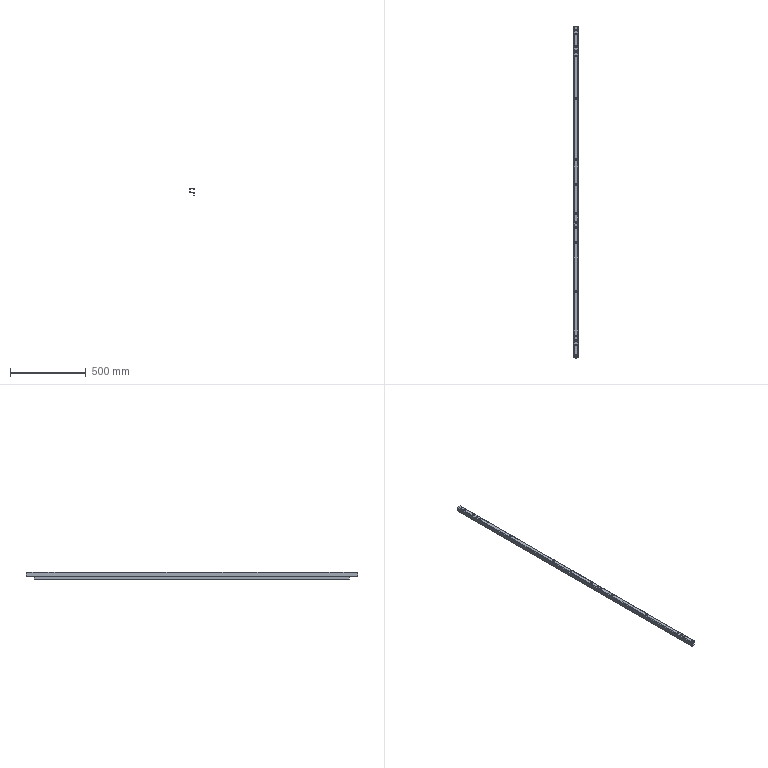Part | NX | features solid 2 | 1 solid | 333 faces | box 27.88 x 2190 x 52.5 mm | volume 578008 mm3 | plane 229 | cylinder 102 | torus 2 | commonest cylinder face diameters 2.5 x33 7.5 x33 11.1 x16 13.1 x14 4 x2 5.3 x2